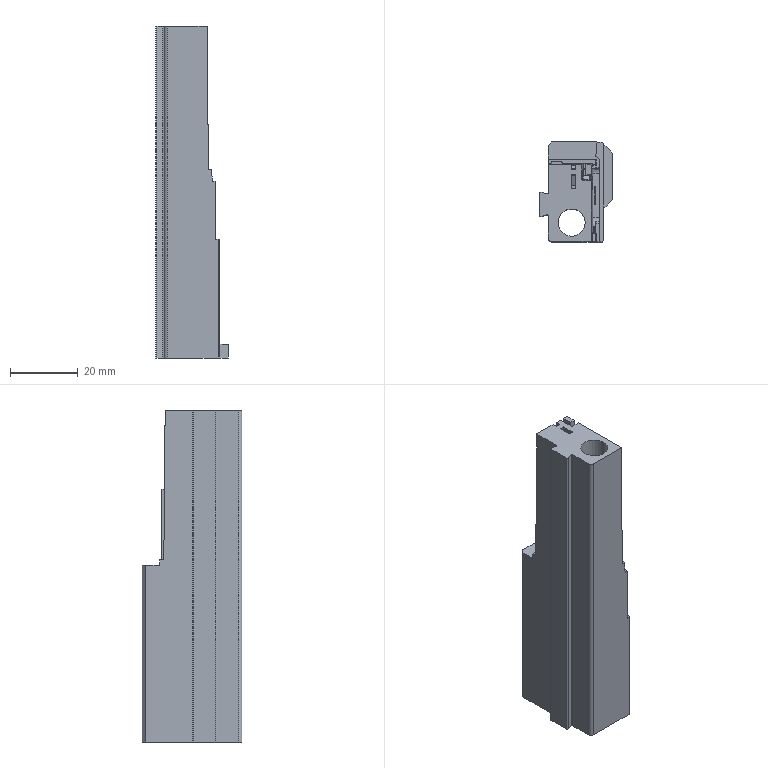Part | Creo | 1 solid | 249 faces | box 21.5 x 29.5 x 98.191 mm | volume 33595 mm3 | plane 130 | other 80 | cylinder 35 | sphere 4 | commonest cylinder face diameters 0.402 x11 0.603 x7 0.6 x4 3.1 x2 3.2 x2 5.166 x2